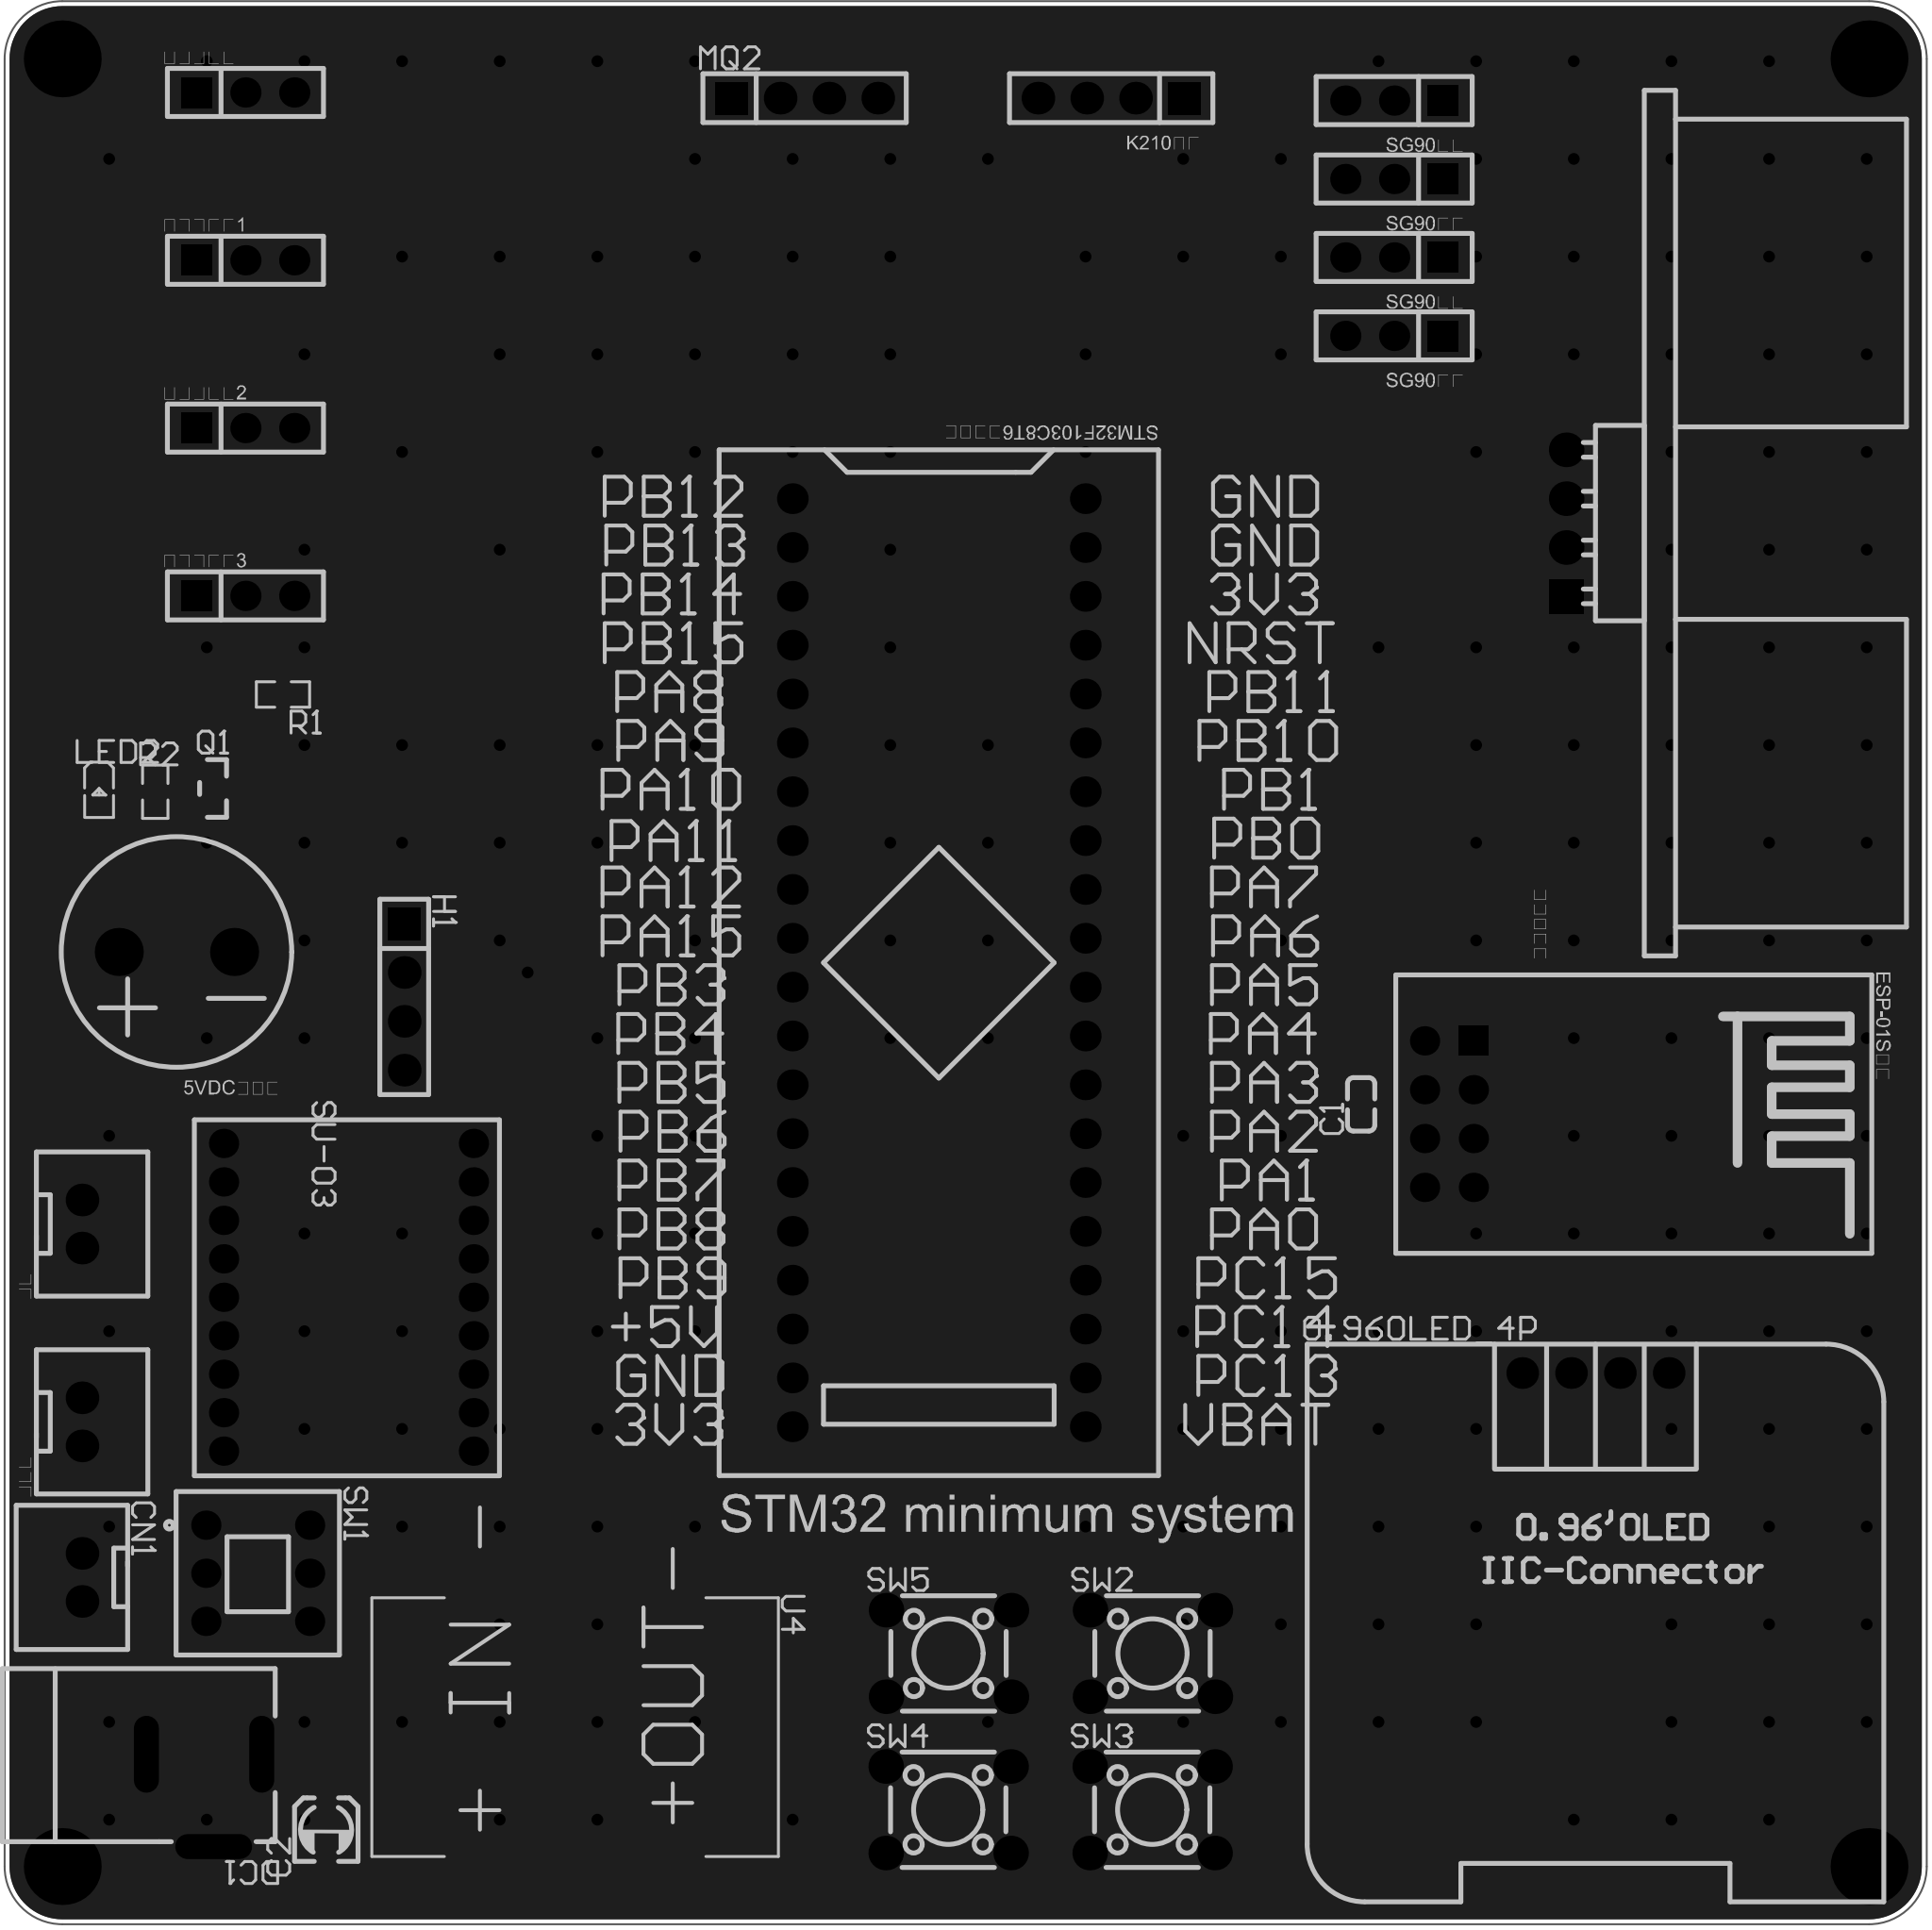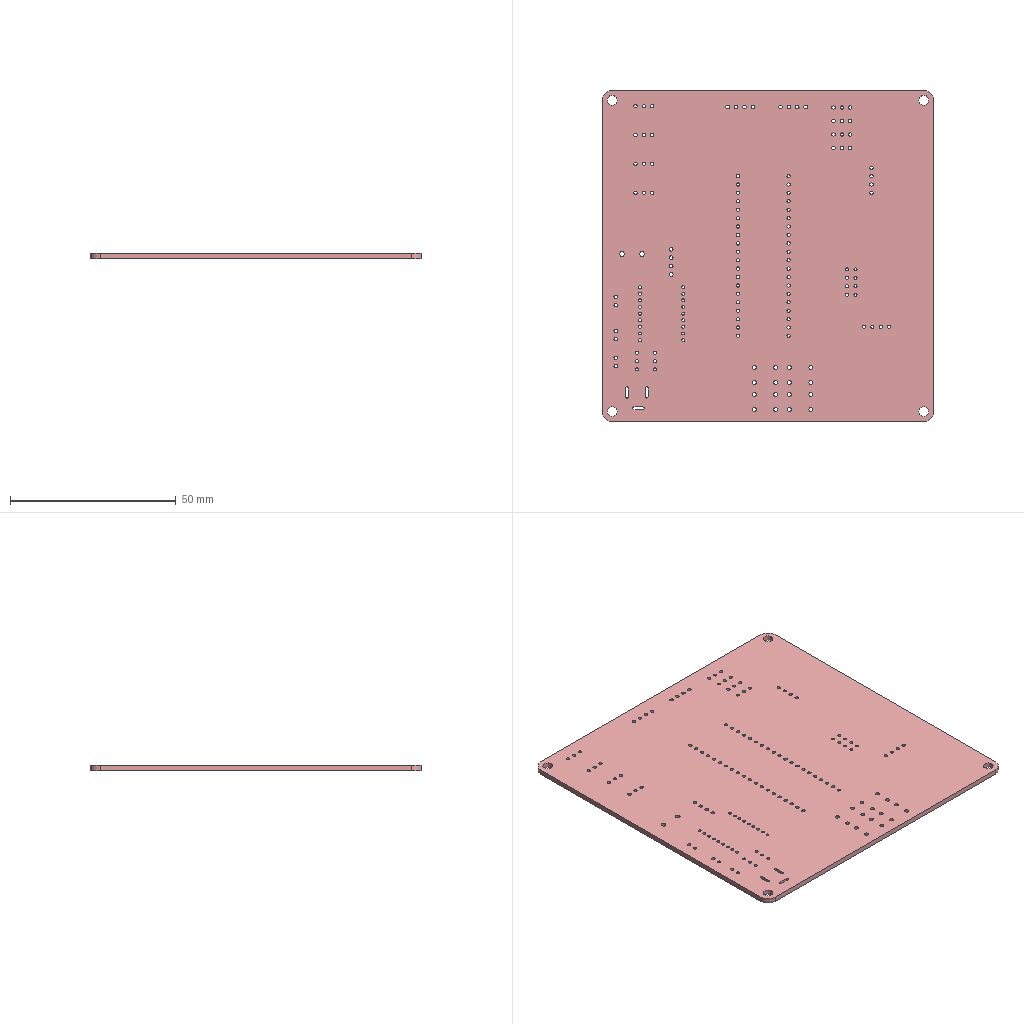Circuit board layout | Altium Designer | box 100 x 100 x 1.6 mm
Layer stack:
# Altium Designer layer stack of  (unit mm; dielectric type: 0 none, 1 core, 2 prepreg, 3 surface material)
index,name,kind,layer,copper_thickness_mm,dielectric_type,dielectric_thickness_mm,dielectric_material,dielectric_constant
0,Top Paste Mask Layer,other,,,,,,
1,Top Silkscreen Layer,other,,,,,,
2,Top Solder Mask Layer,dielectric,,,3,0.01,,3.3
3,Top Layer,copper,Top Layer,0.035,,,,
4,Dielectric1,dielectric,,,3,1.51,FR4,4.5
5,Bottom Layer,copper,Bottom Layer,0.035,,,,
6,Bottom Solder Mask Layer,dielectric,,,3,0.01,,3.3
7,Bottom Silkscreen Layer,other,,,,,,
8,Bottom Paste Mask Layer,other,,,,,,
# drill layer pairs: low layer,high layer
drill_pair,Top Layer,Bottom Layer
Part placement:
Designator,Comment,Layer,Footprint,Center-X(mm),Center-Y(mm),Rotation
STM32F103C8T6最小系统,STM32F103C8T6-Card,TopLayer,CONN-TH_L53.3-W22.9_STM32F103C8T6-CARD,129.159,128.905,270
5VDC蜂鸣器,buzzer,TopLayer,BUZ-TH_BD12.0-P6.00-D0.9-RD,89.496,129.464,180
C1,1uF,TopLayer,C0603,151.13,121.539,90
LED2,,TopLayer,LED_0603,85.463,137.846,270
Q1,,TopLayer,S8050_SOT-23,91.401,137.966,180
R1,1K,TopLayer,R0603,95.038,142.852,180
R2,10K,TopLayer,R0603,88.392,137.795,90
ESP-01S模块,ESP8266-01S,TopLayer,WIFIM-TH_ESP8266-01S,155.702,121.031,270
SU-03,CON2.0MM-PAD-18,TopLayer,CONN-TH_18P-P2.00_C9900078766,98.448,111.506,270
麦克风,XH2.54*2P_through-hole,TopLayer,CONN-TH_2P-P2.50-XH2.54-2P,84.582,105.029,90
喇叭,XH2.54*2P_through-hole,TopLayer,CONN-TH_2P-P2.50-XH2.54-2P,84.582,115.316,90
0.96OLED_4P,,TopLayer,0.96OLED_4P,163.322,107.569,0
C2,1uF,TopLayer,C_Ele_SMD_3x5.4mm,97.296,83.825,90
CN1,XH2.54*2P_through-hole,TopLayer,CONN-TH_2P-P2.50-XH2.54-2P,84.582,96.941,270
DC1,,TopLayer,DC-2.0,90.932,85.344,180
H1,,TopLayer,HDR-TH_4P-P2.54-V-M,101.346,127.127,270
K210接口,,TopLayer,HDR-TH_4P-P2.54-V-F,138.126,173.863,180
MQ2,,TopLayer,HDR-TH_4P-P2.54-V-F,122.174,173.863,0
SG90舵机,,TopLayer,HDR-TH_3P-P2.54-V-F,152.848,161.5,180
SG90舵机,,TopLayer,HDR-TH_3P-P2.54-V-F,152.848,169.657,180
SG90舵机,,TopLayer,HDR-TH_3P-P2.54-V-F,152.848,165.579,180
SG90舵机,,TopLayer,HDR-TH_3P-P2.54-V-F,152.848,173.736,180
SW1,TK-6850-1,TopLayer,SW-TH_TK-6850-1,93.726,97.155,270
SW2,,TopLayer,SW-TH_4P-L6.0-W6.0-P4.50-LS6.5,140.275,92.986,0
SW3,,TopLayer,SW-TH_4P-L6.0-W6.0-P4.50-LS6.5,140.26,84.858,0
SW4,,TopLayer,SW-TH_4P-L6.0-W6.0-P4.50-LS6.5,129.647,84.858,0
SW5,,TopLayer,SW-TH_4P-L6.0-W6.0-P4.50-LS6.5,129.663,92.986,0
U4,,TopLayer,JYMK,110.236,89.154,270
红外传感器,,TopLayer,HDR-TH_3P-P2.54-V-F,93.085,174.158,0
红外传感器1,,TopLayer,HDR-TH_3P-P2.54-V-F,93.085,165.432,0
红外传感器2,,TopLayer,HDR-TH_3P-P2.54-V-F,93.085,156.706,0
红外传感器3,,TopLayer,HDR-TH_3P-P2.54-V-F,93.085,147.98,0
超声波模块,HC-SR04,TopLayer,TH_HC-SR04V,161.798,151.765,90
Pad and via stacks:
# Altium Designer via and pad stacks of  (unit mm). Each distinct definition once, with the count of objects using it.
# via: kind,start_layer,end_layer,hole_mm,diameter_mm,mode(0 simple;1 top-mid-bottom;2 full stack),diameter_per_layer,count,example_net
# pad: kind,layer,hole_mm,hole_type(0 round;1 square;2 slot),plating,top_size,top_shape(1 round;2 rect;3 octagon;9 rounded rect),mid_size,bottom_size,mode,footprint,size_per_layer,count,example
pad,Multi-Layer,3,0,plated,4x4,1,4x4,4x4,0,,,4,1
pad,Multi-Layer,1,0,plated,1.6x1.6,1,1.6x1.6,1.6x1.6,0,CONN-TH_L53.3-W22.9_STM32F103C8T6-CARD,,40,STM32F103C8T6\u6700\u5C0F\u7CFB\u7EDF.1
pad,Multi-Layer,1.5,0,plated,2.5x2.5,1,2.5x2.5,2.5x2.5,0,BUZ-TH_BD12.0-P6.00-D0.9-RD,,2,5VDC\u8702\u9E23\u5668.1
pad,Multi-Layer,0.9144,0,plated,1.524x1.524,1,1.524x1.524,1.524x1.524,0,WIFIM-TH_ESP8266-01S,,7,ESP-01S\u6A21\u5757.8
pad,Multi-Layer,0.9144,0,plated,1.524x1.524,2,1.524x1.524,1.524x1.524,0,WIFIM-TH_ESP8266-01S,,1,ESP-01S\u6A21\u5757.1
pad,Multi-Layer,0.9,0,plated,1.524x1.524,1,1.524x1.524,1.524x1.524,0,CONN-TH_18P-P2.00_C9900078766,,18,SU-03.1
pad,Multi-Layer,1.05,0,plated,1.7x1.7,1,1.7x1.7,1.7x1.7,0,CONN-TH_2P-P2.50-XH2.54-2P,,6,\u9EA6\u514B\u98CE.2
pad,Multi-Layer,1,0,plated,1.65x1.65,1,1.65x1.65,1.65x1.65,0,0.96OLED_4P,,4,0.96OLED_4P.4
pad,Multi-Layer,0.8001,2,plated,4x1.3,1,4x1.3,4x1.3,0,DC-2.0,,3,DC1.2
pad,Multi-Layer,1.1,0,plated,1.7x1.7,2,1.7x1.7,1.7x1.7,0,HDR-TH_4P-P2.54-V-M,,1,H1.1
pad,Multi-Layer,1.1,0,plated,1.7x1.7,1,1.7x1.7,1.7x1.7,0,HDR-TH_4P-P2.54-V-M,,3,H1.2
pad,Multi-Layer,1.1,0,plated,1.7x1.7,2,1.7x1.7,1.7x1.7,0,HDR-TH_4P-P2.54-V-F,,2,K210\u63A5\u53E3.1
pad,Multi-Layer,1.1,0,plated,1.7x1.7,1,1.7x1.7,1.7x1.7,0,HDR-TH_4P-P2.54-V-F,,6,K210\u63A5\u53E3.2
pad,Multi-Layer,1.02,0,plated,1.575x1.575,1,1.575x1.575,1.575x1.575,0,HDR-TH_3P-P2.54-V-F,,16,SG90\u8235\u673A.3
pad,Multi-Layer,1.02,0,plated,1.575x1.575,2,1.575x1.575,1.575x1.575,0,HDR-TH_3P-P2.54-V-F,,8,SG90\u8235\u673A.1
pad,Multi-Layer,0.914,0,plated,1.524x1.524,1,1.524x1.524,1.524x1.524,0,SW-TH_TK-6850-1,,3,SW1.1
pad,Multi-Layer,0.9144,0,plated,1.524x1.524,1,1.524x1.524,1.524x1.524,0,SW-TH_TK-6850-1,,3,SW1.4
pad,Multi-Layer,1.2,0,plated,1.8x1.8,1,1.8x1.8,1.8x1.8,0,SW-TH_4P-L6.0-W6.0-P4.50-LS6.5,,16,SW2.1
pad,Multi-Layer,1.001,0,plated,1.8x1.8,1,1.8x1.8,1.8x1.8,0,TH_HC-SR04V,,3,\u8D85\u58F0\u6CE2\u6A21\u5757.4
pad,Multi-Layer,1.001,0,plated,1.8x1.8,2,1.8x1.8,1.8x1.8,0,TH_HC-SR04V,,1,\u8D85\u58F0\u6CE2\u6A21\u5757.1
pad,Top Layer,0,0,plated,0.8x0.9,2,0.8x0.9,0.8x0.9,0,C0603,,2,C1.2
pad,Top Layer,0,0,plated,0.8001x0.8001,2,0.8001x0.8001,0.8001x0.8001,0,LED_0603,,2,LED2.1
pad,Top Layer,0,0,plated,1x0.8,2,1x0.8,1x0.8,0,S8050_SOT-23,,3,Q1.2
pad,Top Layer,0,0,plated,0.8065x0.864,2,0.8065x0.864,0.8065x0.864,0,R0603,,4,R1.2
pad,Top Layer,0,0,plated,1.999x0.8001,2,1.999x0.8001,1.999x0.8001,0,C_Ele_SMD_3x5.4mm,,2,C2.1
pad,Top Layer,0,0,plated,3.625x2.25,2,3.625x2.25,3.625x2.25,0,JYMK,,4,U4.1
via,Top Layer,Bottom Layer,0.3048,0.61,0,,207,PA9
Copper pours:
name,layer,net,type(0 solid;1 hatched;2 none)
Bottom Layer-GND,Bottom Layer,GND,0
Top Layer-GND,Top Layer,GND,0
Design rules, without the lines most boards share:
# Altium Designer design rules of  (exported by Altium Designer, unit mm)
# columns: name | kind | enabled | priority | scope1 | scope2 | descriptor | typed fields (field=value)
copperThickness1oz_2 | 2 | enabled | 2 | All | All | Width Constraint (Min=5mil) (Max=100mil) (Preferred=30mil) (All) |
viaSize | 11 | enabled | 1 | All | All | Routing Via (MinHoleWidth=11.811mil) (MaxHoleWidth=248.032mil) (PreferredHoleWidth=12.008mil) (MinWidth=19.685mil) (MaxWidth=393.701mil) (PreferedWidth=24.016mil) (All) | via_min_hole=0.3 via_max_hole=6.3 via_preferred_diameter=0.61 via_preferred_hole=0.305
solderMaskExpansion | 13 | enabled | 2 | All | All | Solder Mask Expansion (Expansion =2.008mil) (All) | expansion=0.051